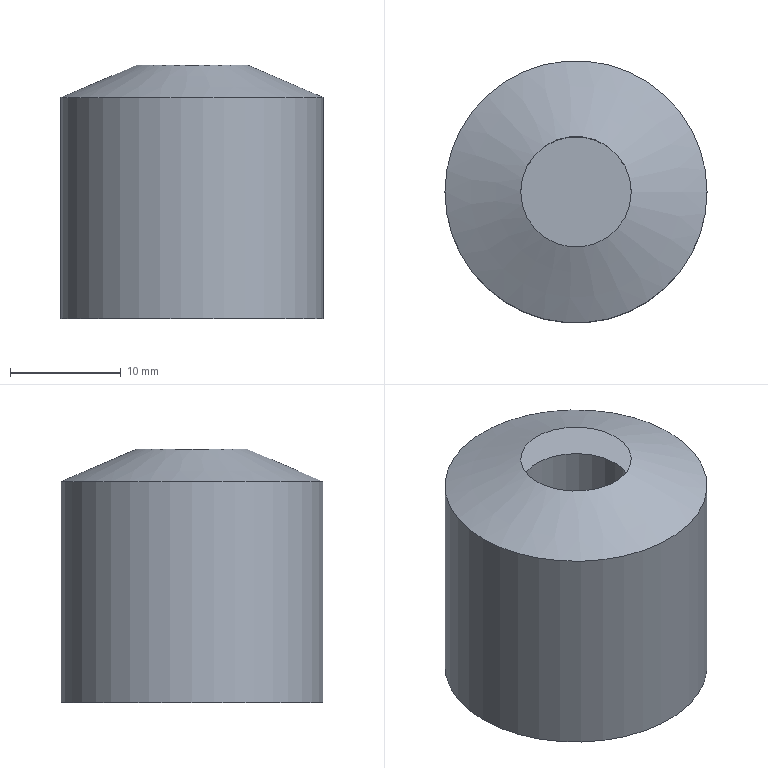Part | NX | features DATUM_PLANE 2, EXTRUDE 2, DATUM_CSYS 1, LINKED_FACE 1, TRIM BODY 1 | 1 solid | 6 faces | box 23.68 x 23.68 x 22.932 mm | volume 5989 mm3 | plane 3 | cylinder 2 | cone 1 | commonest cylinder face diameters 10 x1 23.68 x1